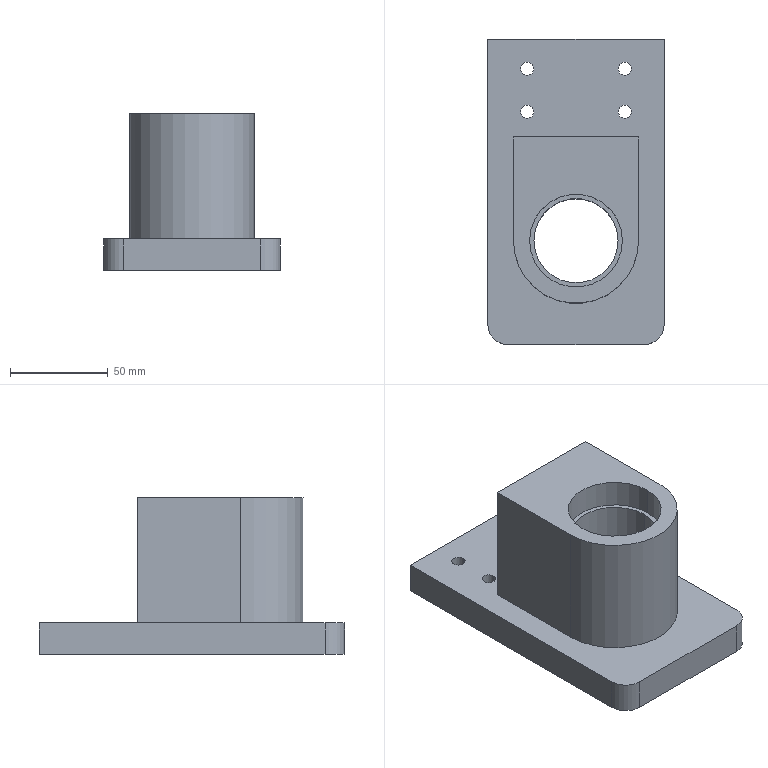NC program | NX | posted with a generic post | part box 90 x 156 x 80 mm
Lines 4832 to 5953 of 8711:
(CAVITY_MILL , TOOL : 刀杆C25-D25-150-2T)
N9656 T01 M6
N9658 G53
N9660 G17 G0 G90 X-99. Y0. S2000 M3
N9662 G43 Z30. H1
N9664 Z-38.5
N9666 G94 G1 Z-40.5 F3000.
N9668 X-82.75
N9670 Y48.792
N9672 X-82.741 Y50.037
N9674 G2 X-81.527 Y51.242 R1.214
N9676 G1 X81.527
N9678 G2 X82.741 Y50.036 R1.214
N9680 G1 X82.749 Y48.794
N9682 Y28.528
N9684 X64.029
N9686 G3 X60.769 Y32.522 R48.344
N9688 G1 X64.029
N9690 Y28.528
N9692 X70.622 Y17.418
N9694 X64.029 Y28.528
N9696 X82.749
N9698 X82.75 Y-48.792
N9700 X82.741 Y-50.037
N9702 G2 X81.527 Y-51.242 R1.214
N9704 G1 X60.769
N9706 Y-32.522
N9708 G3 X64.03 Y-28.527 R48.344
N9710 G1 X70.622 Y-17.417
N9712 X64.03 Y-28.527
N9714 Y-32.522
N9716 X60.769
N9718 Y-51.242
N9720 X-81.527
N9722 G2 X-82.741 Y-50.036 R1.214
N9724 G1 X-82.749 Y-48.794
N9726 X-82.75 Y0.
N9728 X-64.03
N9730 Y32.522
N9732 X-44.336
N9734 G3 X-44.344 Y32. R16.344
N9736 G1 Y-32.
N9738 G3 X-44.336 Y-32.522 R16.344
N9740 G1 X-40.594 Y-32.403
N9742 G2 X-40.6 Y-32. R12.6
N9744 G1 Y32.
N9746 G2 X-28. Y44.6 R12.6
N9748 G1 X25.
N9750 G2 X69.6 Y0. R44.6
N9752 X25. Y-44.6 R44.6
N9754 G1 X-28.
N9756 G2 X-40.594 Y-32.403 R12.6
N9758 G1 X-44.336 Y-32.522
N9760 X-64.029
N9762 X-64.03 Y0.
N9764 X-99.
N9766 Z-38.5
N9768 G0 Z30.
N9770 X33.853 Y-0.916
N9772 Z-37.
N9774 G2 X25. Y-8.9 Z-40.5 R8.9
N9776 X16.1 Y0. R8.9
N9778 X25. Y-8.9 R-8.9
N9780 G1 Z-38.5
N9782 G0 Z-37.5
N9784 X33.853 Y-0.916
N9786 G2 X25. Y-8.9 Z-41. R8.9
N9788 X16.1 Y0. R8.9
N9790 X25. Y-8.9 R-8.9
N9792 G1 Z-39.
N9794 G0 Z30.
N9796 X-99. Y0.
N9798 Z-39.
N9800 G1 Z-41.
N9802 X-82.75
N9804 Y48.792
N9806 X-82.741 Y50.037
N9808 G2 X-81.527 Y51.242 R1.214
N9810 G1 X81.527
N9812 G2 X82.741 Y50.036 R1.214
N9814 G1 X82.749 Y48.794
N9816 Y28.528
N9818 X64.029
N9820 G3 X60.769 Y32.522 R48.344
N9822 G1 X64.029
N9824 Y28.528
N9826 X70.622 Y17.418
N9828 X64.029 Y28.528
N9830 X82.749
N9832 X82.75 Y-48.792
N9834 X82.741 Y-50.037
N9836 G2 X81.527 Y-51.242 R1.214
N9838 G1 X60.769
N9840 Y-32.522
N9842 G3 X64.03 Y-28.527 R48.344
N9844 G1 X70.622 Y-17.417
N9846 X64.03 Y-28.527
N9848 Y-32.522
N9850 X60.769
N9852 Y-51.242
N9854 X-81.527
N9856 G2 X-82.741 Y-50.036 R1.214
N9858 G1 X-82.749 Y-48.794
N9860 X-82.75 Y0.
N9862 X-64.03
N9864 Y32.522
N9866 X-44.336
N9868 G3 X-44.344 Y32. R16.344
N9870 G1 Y-32.
N9872 G3 X-44.336 Y-32.522 R16.344
N9874 G1 X-40.594 Y-32.403
N9876 G2 X-40.6 Y-32. R12.6
N9878 G1 Y32.
N9880 G2 X-28. Y44.6 R12.6
N9882 G1 X25.
N9884 G2 X69.6 Y0. R44.6
N9886 X25. Y-44.6 R44.6
N9888 G1 X-28.
N9890 G2 X-40.594 Y-32.403 R12.6
N9892 G1 X-44.336 Y-32.522
N9894 X-64.029
N9896 X-64.03 Y0.
N9898 X-99.
N9900 Z-39.
N9902 G0 Z-38.5
N9904 Z-39.5
N9906 G1 Z-41.5
N9908 X-82.75
N9910 Y48.792
N9912 X-82.741 Y50.037
N9914 G2 X-81.527 Y51.242 R1.214
N9916 G1 X81.527
N9918 G2 X82.741 Y50.036 R1.214
N9920 G1 X82.749 Y48.794
N9922 Y28.528
N9924 X64.029
N9926 G3 X60.769 Y32.522 R48.344
N9928 G1 X64.029
N9930 Y28.528
N9932 X70.622 Y17.418
N9934 X64.029 Y28.528
N9936 X82.749
N9938 X82.75 Y-48.792
N9940 X82.741 Y-50.037
N9942 G2 X81.527 Y-51.242 R1.214
N9944 G1 X60.769
N9946 Y-32.522
N9948 G3 X64.03 Y-28.527 R48.344
N9950 G1 X70.622 Y-17.417
N9952 X64.03 Y-28.527
N9954 Y-32.522
N9956 X60.769
N9958 Y-51.242
N9960 X-81.527
N9962 G2 X-82.741 Y-50.036 R1.214
N9964 G1 X-82.749 Y-48.794
N9966 X-82.75 Y0.
N9968 X-64.03
N9970 Y32.522
N9972 X-44.336
N9974 G3 X-44.344 Y32. R16.344
N9976 G1 Y-32.
N9978 G3 X-44.336 Y-32.522 R16.344
N9980 G1 X-40.594 Y-32.403
N9982 G2 X-40.6 Y-32. R12.6
N9984 G1 Y32.
N9986 G2 X-28. Y44.6 R12.6
N9988 G1 X25.
N9990 G2 X69.6 Y0. R44.6
N9992 X25. Y-44.6 R44.6
N9994 G1 X-28.
N9996 G2 X-40.594 Y-32.403 R12.6
N9998 G1 X-44.336 Y-32.522
N10000 X-64.029
N10002 X-64.03 Y0.
N10004 X-99.
N10006 Z-39.5
N10008 G0 Z30.
N10010 X33.853 Y-0.916
N10012 Z-38.
N10014 G2 X25. Y-8.9 Z-41.5 R8.9
N10016 X16.1 Y0. R8.9
N10018 X25. Y-8.9 R-8.9
N10020 G1 Z-39.5
N10022 G0 Z-38.5
N10024 X33.853 Y-0.916
N10026 G2 X25. Y-8.9 Z-42. R8.9
N10028 X16.1 Y0. R8.9
N10030 X25. Y-8.9 R-8.9
N10032 G1 Z-40.
N10034 G0 Z30.
N10036 X-99. Y0.
N10038 Z-40.
N10040 G1 Z-42.
N10042 X-82.75
N10044 Y48.792
N10046 X-82.741 Y50.037
N10048 G2 X-81.527 Y51.242 R1.214
N10050 G1 X81.527
N10052 G2 X82.741 Y50.036 R1.214
N10054 G1 X82.749 Y48.794
N10056 Y28.528
N10058 X64.029
N10060 G3 X60.769 Y32.522 R48.344
N10062 G1 X64.029
N10064 Y28.528
N10066 X70.622 Y17.418
N10068 X64.029 Y28.528
N10070 X82.749
N10072 X82.75 Y-48.792
N10074 X82.741 Y-50.037
N10076 G2 X81.527 Y-51.242 R1.214
N10078 G1 X60.769
N10080 Y-32.522
N10082 G3 X64.03 Y-28.527 R48.344
N10084 G1 X70.622 Y-17.417
N10086 X64.03 Y-28.527
N10088 Y-32.522
N10090 X60.769
N10092 Y-51.242
N10094 X-81.527
N10096 G2 X-82.741 Y-50.036 R1.214
N10098 G1 X-82.749 Y-48.794
N10100 X-82.75 Y0.
N10102 X-64.03
N10104 Y32.522
N10106 X-44.336
N10108 G3 X-44.344 Y32. R16.344
N10110 G1 Y-32.
N10112 G3 X-44.336 Y-32.522 R16.344
N10114 G1 X-40.594 Y-32.403
N10116 G2 X-40.6 Y-32. R12.6
N10118 G1 Y32.
N10120 G2 X-28. Y44.6 R12.6
N10122 G1 X25.
N10124 G2 X69.6 Y0. R44.6
N10126 X25. Y-44.6 R44.6
N10128 G1 X-28.
N10130 G2 X-40.594 Y-32.403 R12.6
N10132 G1 X-44.336 Y-32.522
N10134 X-64.029
N10136 X-64.03 Y0.
N10138 X-99.
N10140 Z-40.
N10142 G0 Z-39.5
N10144 Z-40.5
N10146 G1 Z-42.5
N10148 X-82.75
N10150 Y48.792
N10152 X-82.741 Y50.037
N10154 G2 X-81.527 Y51.242 R1.214
N10156 G1 X81.527
N10158 G2 X82.741 Y50.036 R1.214
N10160 G1 X82.749 Y48.794
N10162 Y28.528
N10164 X64.029
N10166 G3 X60.769 Y32.522 R48.344
N10168 G1 X64.029
N10170 Y28.528
N10172 X70.622 Y17.418
N10174 X64.029 Y28.528
N10176 X82.749
N10178 X82.75 Y-48.792
N10180 X82.741 Y-50.037
N10182 G2 X81.527 Y-51.242 R1.214
N10184 G1 X60.769
N10186 Y-32.522
N10188 G3 X64.03 Y-28.527 R48.344
N10190 G1 X70.622 Y-17.417
N10192 X64.03 Y-28.527
N10194 Y-32.522
N10196 X60.769
N10198 Y-51.242
N10200 X-81.527
N10202 G2 X-82.741 Y-50.036 R1.214
N10204 G1 X-82.749 Y-48.794
N10206 X-82.75 Y0.
N10208 X-64.03
N10210 Y32.522
N10212 X-44.336
N10214 G3 X-44.344 Y32. R16.344
N10216 G1 Y-32.
N10218 G3 X-44.336 Y-32.522 R16.344
N10220 G1 X-40.594 Y-32.403
N10222 G2 X-40.6 Y-32. R12.6
N10224 G1 Y32.
N10226 G2 X-28. Y44.6 R12.6
N10228 G1 X25.
N10230 G2 X69.6 Y0. R44.6
N10232 X25. Y-44.6 R44.6
N10234 G1 X-28.
N10236 G2 X-40.594 Y-32.403 R12.6
N10238 G1 X-44.336 Y-32.522
N10240 X-64.029
N10242 X-64.03 Y0.
N10244 X-99.
N10246 Z-40.5
N10248 G0 Z30.
N10250 X33.853 Y-0.916
N10252 Z-39.
N10254 G2 X25. Y-8.9 Z-42.5 R8.9
N10256 X16.1 Y0. R8.9
N10258 X25. Y-8.9 R-8.9
N10260 G1 Z-40.5
N10262 G0 Z-39.5
N10264 X33.853 Y-0.916
N10266 G2 X25. Y-8.9 Z-43. R8.9
N10268 X16.1 Y0. R8.9
N10270 X25. Y-8.9 R-8.9
N10272 G1 Z-41.
N10274 G0 Z30.
N10276 X-99. Y0.
N10278 Z-41.
N10280 G1 Z-43.
N10282 X-82.75
N10284 Y48.792
N10286 X-82.741 Y50.037
N10288 G2 X-81.527 Y51.242 R1.214
N10290 G1 X81.527
N10292 G2 X82.741 Y50.036 R1.214
N10294 G1 X82.749 Y48.794
N10296 Y28.528
N10298 X64.029
N10300 G3 X60.769 Y32.522 R48.344
N10302 G1 X64.029
N10304 Y28.528
N10306 X70.622 Y17.418
N10308 X64.029 Y28.528
N10310 X82.749
N10312 X82.75 Y-48.792
N10314 X82.741 Y-50.037
N10316 G2 X81.527 Y-51.242 R1.214
N10318 G1 X60.769
N10320 Y-32.522
N10322 G3 X64.03 Y-28.527 R48.344
N10324 G1 X70.622 Y-17.417
N10326 X64.03 Y-28.527
N10328 Y-32.522
N10330 X60.769
N10332 Y-51.242
N10334 X-81.527
N10336 G2 X-82.741 Y-50.036 R1.214
N10338 G1 X-82.749 Y-48.794
N10340 X-82.75 Y0.
N10342 X-64.03
N10344 Y32.522
N10346 X-44.336
N10348 G3 X-44.344 Y32. R16.344
N10350 G1 Y-32.
N10352 G3 X-44.336 Y-32.522 R16.344
N10354 G1 X-40.594 Y-32.403
N10356 G2 X-40.6 Y-32. R12.6
N10358 G1 Y32.
N10360 G2 X-28. Y44.6 R12.6
N10362 G1 X25.
N10364 G2 X69.6 Y0. R44.6
N10366 X25. Y-44.6 R44.6
N10368 G1 X-28.
N10370 G2 X-40.594 Y-32.403 R12.6
N10372 G1 X-44.336 Y-32.522
N10374 X-64.029
N10376 X-64.03 Y0.
N10378 X-99.
N10380 Z-41.
N10382 G0 Z-40.5
N10384 Z-41.5
N10386 G1 Z-43.5
N10388 X-82.75
N10390 Y48.792
N10392 X-82.741 Y50.037
N10394 G2 X-81.527 Y51.242 R1.214
N10396 G1 X81.527
N10398 G2 X82.741 Y50.036 R1.214
N10400 G1 X82.749 Y48.794
N10402 X82.75 Y28.528
N10404 X64.03
N10406 G3 X60.769 Y32.522 R48.344
N10408 G1 X64.029
N10410 X64.03 Y28.528
N10412 X70.622 Y17.418
N10414 X64.03 Y28.528
N10416 X82.75
N10418 Y-48.792
N10420 X82.741 Y-50.037
N10422 G2 X81.527 Y-51.242 R1.214
N10424 G1 X60.769
N10426 Y-32.522
N10428 G3 X64.03 Y-28.527 R48.344
N10430 G1 X70.622 Y-17.417
N10432 X64.03 Y-28.527
N10434 Y-32.522
N10436 X60.769
N10438 Y-51.242
N10440 X-81.527
N10442 G2 X-82.741 Y-50.036 R1.214
N10444 G1 X-82.749 Y-48.794
N10446 X-82.75 Y0.
N10448 X-64.03
N10450 Y32.522
N10452 X-44.336
N10454 G3 X-44.344 Y32. R16.344
N10456 G1 Y-32.
N10458 G3 X-44.336 Y-32.522 R16.344
N10460 G1 X-40.594 Y-32.403
N10462 G2 X-40.6 Y-32. R12.6
N10464 G1 Y32.
N10466 G2 X-28. Y44.6 R12.6
N10468 G1 X25.
N10470 G2 X69.6 Y0. R44.6
N10472 X25. Y-44.6 R44.6
N10474 G1 X-28.
N10476 G2 X-40.594 Y-32.403 R12.6
N10478 G1 X-44.336 Y-32.522
N10480 X-64.029
N10482 X-64.03 Y0.
N10484 X-99.
N10486 Z-41.5
N10488 G0 Z30.
N10490 X33.853 Y-0.916
N10492 Z-40.
N10494 G2 X25. Y-8.9 Z-43.5 R8.9
N10496 X16.1 Y0. R8.9
N10498 X25. Y-8.9 R-8.9
N10500 G1 Z-41.5
N10502 G0 Z-40.5
N10504 X33.853 Y-0.916
N10506 G2 X25. Y-8.9 Z-44. R8.9
N10508 X16.1 Y0. R8.9
N10510 X25. Y-8.9 R-8.9
N10512 G1 Z-42.
N10514 G0 Z30.
N10516 X-99. Y0.
N10518 Z-42.
N10520 G1 Z-44.
N10522 X-82.75
N10524 Y48.792
N10526 X-82.741 Y50.037
N10528 G2 X-81.527 Y51.242 R1.214
N10530 G1 X81.527
N10532 G2 X82.741 Y50.036 R1.214
N10534 G1 X82.749 Y48.794
N10536 X82.75 Y28.528
N10538 X64.03
N10540 G3 X60.769 Y32.522 R48.344
N10542 G1 X64.029
N10544 X64.03 Y28.528
N10546 X70.622 Y17.418
N10548 X64.03 Y28.528
N10550 X82.75
N10552 Y-48.792
N10554 X82.741 Y-50.037
N10556 G2 X81.527 Y-51.242 R1.214
N10558 G1 X60.769
N10560 Y-32.522
N10562 G3 X64.03 Y-28.527 R48.344
N10564 G1 X70.622 Y-17.417
N10566 X64.03 Y-28.527
N10568 Y-32.522
N10570 X60.769
N10572 Y-51.242
N10574 X-81.527
N10576 G2 X-82.741 Y-50.036 R1.214
N10578 G1 X-82.749 Y-48.794
N10580 X-82.75 Y0.
N10582 X-64.03
N10584 Y32.522
N10586 X-44.336
N10588 G3 X-44.344 Y32. R16.344
N10590 G1 Y-32.
N10592 G3 X-44.336 Y-32.522 R16.344
N10594 G1 X-40.594 Y-32.403
N10596 G2 X-40.6 Y-32. R12.6
N10598 G1 Y32.
N10600 G2 X-28. Y44.6 R12.6
N10602 G1 X25.
N10604 G2 X69.6 Y0. R44.6
N10606 X25. Y-44.6 R44.6
N10608 G1 X-28.
N10610 G2 X-40.594 Y-32.403 R12.6
N10612 G1 X-44.336 Y-32.522
N10614 X-64.029
N10616 X-64.03 Y0.
N10618 X-99.
N10620 Z-42.
N10622 G0 Z-41.5
N10624 Z-42.5
N10626 G1 Z-44.5
N10628 X-82.75
N10630 Y48.792
N10632 X-82.741 Y50.037
N10634 G2 X-81.527 Y51.242 R1.214
N10636 G1 X81.527
N10638 G2 X82.741 Y50.036 R1.214
N10640 G1 X82.749 Y48.794
N10642 X82.75 Y28.528
N10644 X64.03
N10646 G3 X60.769 Y32.522 R48.344
N10648 G1 X64.029
N10650 X64.03 Y28.528
N10652 X70.622 Y17.418
N10654 X64.03 Y28.528
N10656 X82.75
N10658 Y-48.792
N10660 X82.741 Y-50.037
N10662 G2 X81.527 Y-51.242 R1.214
N10664 G1 X60.769
N10666 Y-32.522
N10668 G3 X64.03 Y-28.527 R48.344
N10670 G1 X70.622 Y-17.417
N10672 X64.03 Y-28.527
N10674 Y-32.522
N10676 X60.769
N10678 Y-51.242
N10680 X-81.527
N10682 G2 X-82.741 Y-50.036 R1.214
N10684 G1 X-82.749 Y-48.794
N10686 X-82.75 Y0.
N10688 X-64.03
N10690 Y32.522
N10692 X-44.336
N10694 G3 X-44.344 Y32. R16.344
N10696 G1 Y-32.
N10698 G3 X-44.336 Y-32.522 R16.344
N10700 G1 X-40.594 Y-32.403
N10702 G2 X-40.6 Y-32. R12.6
N10704 G1 Y32.
N10706 G2 X-28. Y44.6 R12.6
N10708 G1 X25.
N10710 G2 X69.6 Y0. R44.6
N10712 X25. Y-44.6 R44.6
N10714 G1 X-28.
N10716 G2 X-40.594 Y-32.403 R12.6
N10718 G1 X-44.336 Y-32.522
N10720 X-64.029
N10722 X-64.03 Y0.
N10724 X-99.
N10726 Z-42.5
N10728 G0 Z30.
N10730 X33.853 Y-0.916
N10732 Z-41.
N10734 G2 X25. Y-8.9 Z-44.5 R8.9
N10736 X16.1 Y0. R8.9
N10738 X25. Y-8.9 R-8.9
N10740 G1 Z-42.5
N10742 G0 Z-41.5
N10744 X33.853 Y-0.916
N10746 G2 X25. Y-8.9 Z-45. R8.9
N10748 X16.1 Y0. R8.9
N10750 X25. Y-8.9 R-8.9
N10752 G1 Z-43.
N10754 G0 Z30.
N10756 X-99. Y0.
N10758 Z-43.
N10760 G1 Z-45.
N10762 X-82.75
N10764 Y48.792
N10766 X-82.741 Y50.037
N10768 G2 X-81.527 Y51.242 R1.214
N10770 G1 X81.527
N10772 G2 X82.741 Y50.036 R1.214
N10774 G1 X82.749 Y48.794
N10776 X82.75 Y28.528
N10778 X64.03
N10780 G3 X60.769 Y32.522 R48.344
N10782 G1 X64.029
N10784 X64.03 Y28.528
N10786 X70.622 Y17.418
N10788 X64.03 Y28.528
N10790 X82.75
N10792 Y-48.792
N10794 X82.741 Y-50.037
N10796 G2 X81.527 Y-51.242 R1.214
N10798 G1 X60.769
N10800 Y-32.522
N10802 G3 X64.03 Y-28.527 R48.344
N10804 G1 X70.622 Y-17.417
N10806 X64.03 Y-28.527
N10808 Y-32.522
N10810 X60.769
N10812 Y-51.242
N10814 X-81.527
N10816 G2 X-82.741 Y-50.036 R1.214
N10818 G1 X-82.749 Y-48.794
N10820 X-82.75 Y0.
N10822 X-64.03
N10824 Y32.522
N10826 X-44.336
N10828 G3 X-44.344 Y32. R16.344
N10830 G1 Y-32.
N10832 G3 X-44.336 Y-32.522 R16.344
N10834 G1 X-40.594 Y-32.403
N10836 G2 X-40.6 Y-32. R12.6
N10838 G1 Y32.
N10840 G2 X-28. Y44.6 R12.6
N10842 G1 X25.
N10844 G2 X69.6 Y0. R44.6
N10846 X25. Y-44.6 R44.6
N10848 G1 X-28.
N10850 G2 X-40.594 Y-32.403 R12.6
N10852 G1 X-44.336 Y-32.522
N10854 X-64.029
N10856 X-64.03 Y0.
N10858 X-99.
N10860 Z-43.
N10862 G0 Z-42.5
N10864 Z-43.5
N10866 G1 Z-45.5
N10868 X-82.75
N10870 Y48.792
N10872 X-82.741 Y50.037
N10874 G2 X-81.527 Y51.242 R1.214
N10876 G1 X81.527
N10878 G2 X82.741 Y50.036 R1.214
N10880 G1 X82.749 Y48.794
N10882 X82.75 Y28.528
N10884 X64.03
N10886 G3 X60.769 Y32.522 R48.344
N10888 G1 X64.029
N10890 X64.03 Y28.528
N10892 X70.622 Y17.418
N10894 X64.03 Y28.528
N10896 X82.75
N10898 Y-48.792
N10900 X82.741 Y-50.037
N10902 G2 X81.527 Y-51.242 R1.214
N10904 G1 X60.769
N10906 Y-32.522
N10908 G3 X64.03 Y-28.527 R48.344
N10910 G1 X70.622 Y-17.417
N10912 X64.03 Y-28.527
N10914 Y-32.522
N10916 X60.769
N10918 Y-51.242
N10920 X-81.527
N10922 G2 X-82.741 Y-50.036 R1.214
N10924 G1 X-82.749 Y-48.794
N10926 X-82.75 Y0.
N10928 X-64.03
N10930 Y32.522
N10932 X-44.336
N10934 G3 X-44.344 Y32. R16.344
N10936 G1 Y-32.
N10938 G3 X-44.336 Y-32.522 R16.344
N10940 G1 X-40.594 Y-32.403
N10942 G2 X-40.6 Y-32. R12.6
N10944 G1 Y32.
N10946 G2 X-28. Y44.6 R12.6
N10948 G1 X25.
N10950 G2 X69.6 Y0. R44.6
N10952 X25. Y-44.6 R44.6
N10954 G1 X-28.
N10956 G2 X-40.594 Y-32.403 R12.6
N10958 G1 X-44.336 Y-32.522
N10960 X-64.029
N10962 X-64.03 Y0.
N10964 X-99.
N10966 Z-43.5
N10968 G0 Z30.
N10970 X33.853 Y-0.916
N10972 Z-42.
N10974 G2 X25. Y-8.9 Z-45.5 R8.9
N10976 X16.1 Y0. R8.9
N10978 X25. Y-8.9 R-8.9
N10980 G1 Z-43.5
N10982 G0 Z-42.5
N10984 X33.853 Y-0.916
N10986 G2 X25. Y-8.9 Z-46. R8.9
N10988 X16.1 Y0. R8.9
N10990 X25. Y-8.9 R-8.9
N10992 G1 Z-44.
N10994 G0 Z30.
N10996 X-99. Y0.
N10998 Z-44.
N11000 G1 Z-46.
N11002 X-82.75
N11004 Y48.792
N11006 X-82.741 Y50.037
N11008 G2 X-81.527 Y51.242 R1.214
N11010 G1 X81.527
N11012 G2 X82.741 Y50.036 R1.214
N11014 G1 X82.749 Y48.794
N11016 X82.75 Y28.528
N11018 X64.03
N11020 G3 X60.769 Y32.522 R48.344
N11022 G1 X64.03
N11024 Y28.528
N11026 X70.622 Y17.418
N11028 X64.03 Y28.528
N11030 X82.75
N11032 Y-48.792
N11034 X82.741 Y-50.037
N11036 G2 X81.527 Y-51.242 R1.214
N11038 G1 X60.769
N11040 Y-32.522
N11042 G3 X64.03 Y-28.527 R48.344
N11044 G1 X70.622 Y-17.417
N11046 X64.03 Y-28.527
N11048 Y-32.522
N11050 X60.769
N11052 Y-51.242
N11054 X-81.527
N11056 G2 X-82.741 Y-50.036 R1.214
N11058 G1 X-82.749 Y-48.794
N11060 X-82.75 Y0.
N11062 X-64.03
N11064 Y32.522
N11066 X-44.336
N11068 G3 X-44.344 Y32. R16.344
N11070 G1 Y-32.
N11072 G3 X-44.336 Y-32.522 R16.344
N11074 G1 X-40.594 Y-32.403
N11076 G2 X-40.6 Y-32. R12.6
N11078 G1 Y32.
N11080 G2 X-28. Y44.6 R12.6
N11082 G1 X25.
N11084 G2 X69.6 Y0. R44.6
N11086 X25. Y-44.6 R44.6
N11088 G1 X-28.
N11090 G2 X-40.594 Y-32.403 R12.6
N11092 G1 X-44.336 Y-32.522
N11094 X-64.03
N11096 Y0.
N11098 X-99.
N11100 Z-44.
N11102 G0 Z-43.5
N11104 Z-44.5
N11106 G1 Z-46.5
N11108 X-82.75
N11110 Y48.792
N11112 X-82.741 Y50.037
N11114 G2 X-81.527 Y51.242 R1.214
N11116 G1 X81.527
N11118 G2 X82.741 Y50.036 R1.214
N11120 G1 X82.749 Y48.794
N11122 X82.75 Y28.528
N11124 X64.03
N11126 G3 X60.769 Y32.522 R48.344
N11128 G1 X64.03
N11130 Y28.528
N11132 X70.622 Y17.418
N11134 X64.03 Y28.528
N11136 X82.75
N11138 Y-48.792
N11140 X82.741 Y-50.037
N11142 G2 X81.527 Y-51.242 R1.214
N11144 G1 X60.769
N11146 Y-32.522
N11148 G3 X64.03 Y-28.527 R48.344
N11150 G1 X70.622 Y-17.417
N11152 X64.03 Y-28.527
N11154 Y-32.522
N11156 X60.769
N11158 Y-51.242
N11160 X-81.527
N11162 G2 X-82.741 Y-50.036 R1.214
N11164 G1 X-82.749 Y-48.794
N11166 X-82.75 Y0.
N11168 X-64.03
N11170 Y32.522
N11172 X-44.336
N11174 G3 X-44.344 Y32. R16.344
N11176 G1 Y-32.
N11178 G3 X-44.336 Y-32.522 R16.344
N11180 G1 X-40.594 Y-32.403
N11182 G2 X-40.6 Y-32. R12.6
N11184 G1 Y32.
N11186 G2 X-28. Y44.6 R12.6
N11188 G1 X25.
N11190 G2 X69.6 Y0. R44.6
N11192 X25. Y-44.6 R44.6
N11194 G1 X-28.
N11196 G2 X-40.594 Y-32.403 R12.6
N11198 G1 X-44.336 Y-32.522
N11200 X-64.03
N11202 Y0.
N11204 X-99.
N11206 Z-44.5
N11208 G0 Z30.
N11210 X33.853 Y-0.916
N11212 Z-43.
N11214 G2 X25. Y-8.9 Z-46.5 R8.9
N11216 X16.1 Y0. R8.9
N11218 X25. Y-8.9 R-8.9
N11220 G1 Z-44.5
N11222 G0 Z-43.5
N11224 X33.853 Y-0.916
N11226 G2 X25. Y-8.9 Z-47. R8.9
N11228 X16.1 Y0. R8.9
N11230 X25. Y-8.9 R-8.9
N11232 G1 Z-45.
N11234 G0 Z30.
N11236 X-99. Y0.
N11238 Z-45.
N11240 G1 Z-47.
N11242 X-82.75
N11244 Y48.792
N11246 X-82.741 Y50.037
N11248 G2 X-81.527 Y51.242 R1.214
N11250 G1 X81.527
N11252 G2 X82.741 Y50.036 R1.214
N11254 G1 X82.749 Y48.794
N11256 X82.75 Y28.528
N11258 X64.03
N11260 G3 X60.769 Y32.522 R48.344
N11262 G1 X64.03
N11264 Y28.528
N11266 X70.622 Y17.418
N11268 X64.03 Y28.528
N11270 X82.75
N11272 Y-48.792
N11274 X82.741 Y-50.037
N11276 G2 X81.527 Y-51.242 R1.214
N11278 G1 X60.769
N11280 Y-32.522
N11282 G3 X64.03 Y-28.527 R48.344
N11284 G1 X70.622 Y-17.417
N11286 X64.03 Y-28.527
N11288 Y-32.522
N11290 X60.769
N11292 Y-51.242
N11294 X-81.527
N11296 G2 X-82.741 Y-50.036 R1.214
N11298 G1 X-82.749 Y-48.794
N11300 X-82.75 Y0.
N11302 X-64.03
N11304 Y32.522
N11306 X-44.336
N11308 G3 X-44.344 Y32. R16.344
N11310 G1 Y-32.
N11312 G3 X-44.336 Y-32.522 R16.344
N11314 G1 X-40.594 Y-32.403
N11316 G2 X-40.6 Y-32. R12.6
N11318 G1 Y32.
N11320 G2 X-28. Y44.6 R12.6
N11322 G1 X25.
N11324 G2 X69.6 Y0. R44.6
N11326 X25. Y-44.6 R44.6
N11328 G1 X-28.
N11330 G2 X-40.594 Y-32.403 R12.6
N11332 G1 X-44.336 Y-32.522
N11334 X-64.03
N11336 Y0.
N11338 X-99.
N11340 Z-45.
N11342 G0 Z-44.5
N11344 Z-45.5
N11346 G1 Z-47.5
N11348 X-82.75
N11350 Y48.792
N11352 X-82.741 Y50.037
N11354 G2 X-81.527 Y51.242 R1.214
N11356 G1 X81.527
N11358 G2 X82.741 Y50.036 R1.214
N11360 G1 X82.749 Y48.794
N11362 X82.75 Y28.528
N11364 X64.03
N11366 G3 X60.769 Y32.522 R48.344
N11368 G1 X64.03
N11370 Y28.528
N11372 X70.622 Y17.418
N11374 X64.03 Y28.528
N11376 X82.75
N11378 Y-48.792
N11380 X82.741 Y-50.037
N11382 G2 X81.527 Y-51.242 R1.214
N11384 G1 X60.769
N11386 Y-32.522
N11388 G3 X64.03 Y-28.527 R48.344
N11390 G1 X70.622 Y-17.417
N11392 X64.03 Y-28.527
N11394 Y-32.522
N11396 X60.769
N11398 Y-51.242
N11400 X-81.527
N11402 G2 X-82.741 Y-50.036 R1.214
N11404 G1 X-82.749 Y-48.794
N11406 X-82.75 Y0.
N11408 X-64.03
N11410 Y32.522
N11412 X-44.336
N11414 G3 X-44.344 Y32. R16.344
N11416 G1 Y-32.
N11418 G3 X-44.336 Y-32.522 R16.344
N11420 G1 X-40.594 Y-32.403
N11422 G2 X-40.6 Y-32. R12.6
N11424 G1 Y32.
N11426 G2 X-28. Y44.6 R12.6
N11428 G1 X25.
N11430 G2 X69.6 Y0. R44.6
N11432 X25. Y-44.6 R44.6
N11434 G1 X-28.
N11436 G2 X-40.594 Y-32.403 R12.6
N11438 G1 X-44.336 Y-32.522
N11440 X-64.03
N11442 Y0.
N11444 X-99.
N11446 Z-45.5
N11448 G0 Z30.
N11450 X33.853 Y-0.916
N11452 Z-44.
N11454 G2 X25. Y-8.9 Z-47.5 R8.9
N11456 X16.1 Y0. R8.9
N11458 X25. Y-8.9 R-8.9
N11460 G1 Z-45.5
N11462 G0 Z-44.5
N11464 X33.853 Y-0.916
N11466 G2 X25. Y-8.9 Z-48. R8.9
N11468 X16.1 Y0. R8.9
N11470 X25. Y-8.9 R-8.9
N11472 G1 Z-46.
N11474 G0 Z30.
N11476 X-99. Y0.
N11478 Z-46.
N11480 G1 Z-48.
N11482 X-82.75
N11484 Y48.792
N11486 X-82.741 Y50.037
N11488 G2 X-81.527 Y51.242 R1.214
N11490 G1 X81.527
N11492 G2 X82.741 Y50.036 R1.214
N11494 G1 X82.749 Y48.794
N11496 X82.75 Y28.528
N11498 X64.03
N11500 G3 X60.769 Y32.522 R48.344
N11502 G1 X64.03
N11504 Y28.528
N11506 X70.622 Y17.418
N11508 X64.03 Y28.528
N11510 X82.75
N11512 Y-48.792
N11514 X82.741 Y-50.037
N11516 G2 X81.527 Y-51.242 R1.214
N11518 G1 X60.769
N11520 Y-32.522
N11522 G3 X64.03 Y-28.527 R48.344
N11524 G1 X70.622 Y-17.417
N11526 X64.03 Y-28.527
N11528 Y-32.522
N11530 X60.769
N11532 Y-51.242
N11534 X-81.527
N11536 G2 X-82.741 Y-50.036 R1.214
N11538 G1 X-82.749 Y-48.794
N11540 X-82.75 Y0.
N11542 X-64.03
N11544 Y32.522
N11546 X-44.336
N11548 G3 X-44.344 Y32. R16.344
N11550 G1 Y-32.
N11552 G3 X-44.336 Y-32.522 R16.344
N11554 G1 X-40.594 Y-32.403
N11556 G2 X-40.6 Y-32. R12.6
N11558 G1 Y32.
N11560 G2 X-28. Y44.6 R12.6
N11562 G1 X25.
N11564 G2 X69.6 Y0. R44.6
N11566 X25. Y-44.6 R44.6
N11568 G1 X-28.
N11570 G2 X-40.594 Y-32.403 R12.6
N11572 G1 X-44.336 Y-32.522
N11574 X-64.03
N11576 Y0.
N11578 X-99.
N11580 Z-46.
N11582 G0 Z-45.5
N11584 Z-46.5
N11586 G1 Z-48.5
N11588 X-82.75
N11590 Y48.792
N11592 X-82.741 Y50.037
N11594 G2 X-81.527 Y51.242 R1.214
N11596 G1 X81.527
N11598 G2 X82.741 Y50.036 R1.214
N11600 G1 X82.749 Y48.794
N11602 X82.75 Y28.528
N11604 X64.03
N11606 G3 X60.769 Y32.522 R48.344
N11608 G1 X64.03
N11610 Y28.528
N11612 X70.622 Y17.418
N11614 X64.03 Y28.528
N11616 X82.75
N11618 Y-48.792
N11620 X82.741 Y-50.037
N11622 G2 X81.527 Y-51.242 R1.214
N11624 G1 X60.769
N11626 Y-32.522
N11628 G3 X64.03 Y-28.527 R48.344
N11630 G1 X70.622 Y-17.417
N11632 X64.03 Y-28.527
N11634 Y-32.522
N11636 X60.769
N11638 Y-51.242
N11640 X-81.527
N11642 G2 X-82.741 Y-50.036 R1.214
N11644 G1 X-82.749 Y-48.794
N11646 X-82.75 Y0.
N11648 X-64.03
N11650 Y32.522
N11652 X-44.336
N11654 G3 X-44.344 Y32. R16.344
N11656 G1 Y-32.
N11658 G3 X-44.336 Y-32.522 R16.344
N11660 G1 X-40.594 Y-32.403
N11662 G2 X-40.6 Y-32. R12.6
N11664 G1 Y32.
N11666 G2 X-28. Y44.6 R12.6
N11668 G1 X25.
N11670 G2 X69.6 Y0. R44.6
N11672 X25. Y-44.6 R44.6
N11674 G1 X-28.
N11676 G2 X-40.594 Y-32.403 R12.6
N11678 G1 X-44.336 Y-32.522
N11680 X-64.03
N11682 Y0.
N11684 X-99.
N11686 Z-46.5
N11688 G0 Z30.
N11690 X33.853 Y-0.916
N11692 Z-45.
N11694 G2 X25. Y-8.9 Z-48.5 R8.9
N11696 X16.1 Y0. R8.9
N11698 X25. Y-8.9 R-8.9
N11700 G1 Z-46.5
N11702 G0 Z-45.5
N11704 X33.853 Y-0.916
N11706 G2 X25. Y-8.9 Z-49. R8.9
N11708 X16.1 Y0. R8.9
N11710 X25. Y-8.9 R-8.9
N11712 G1 Z-47.
N11714 G0 Z30.
N11716 X-99. Y0.
N11718 Z-47.
N11720 G1 Z-49.
N11722 X-82.75
N11724 Y48.792
N11726 X-82.741 Y50.037
N11728 G2 X-81.527 Y51.242 R1.214
N11730 G1 X81.527
N11732 G2 X82.741 Y50.036 R1.214
N11734 G1 X82.749 Y48.794
N11736 X82.75 Y28.528
N11738 X64.03
N11740 G3 X60.769 Y32.522 R48.344
N11742 G1 X64.03
N11744 Y28.528
N11746 X70.622 Y17.418
N11748 X64.03 Y28.528
N11750 X82.75
N11752 Y-48.792
N11754 X82.741 Y-50.037
N11756 G2 X81.527 Y-51.242 R1.214
N11758 G1 X60.769
N11760 Y-32.522
N11762 G3 X64.03 Y-28.527 R48.344
N11764 G1 X70.622 Y-17.417
N11766 X64.03 Y-28.527
N11768 Y-32.522
N11770 X60.769
N11772 Y-51.242
N11774 X-81.527
N11776 G2 X-82.741 Y-50.036 R1.214
N11778 G1 X-82.749 Y-48.794
N11780 X-82.75 Y0.
N11782 X-64.03
N11784 Y32.522
N11786 X-44.336
N11788 G3 X-44.344 Y32. R16.344
N11790 G1 Y-32.
N11792 G3 X-44.336 Y-32.522 R16.344
N11794 G1 X-40.594 Y-32.403
N11796 G2 X-40.6 Y-32. R12.6
N11798 G1 Y32.
N11800 G2 X-28. Y44.6 R12.6
N11802 G1 X25.
N11804 G2 X69.6 Y0. R44.6
N11806 X25. Y-44.6 R44.6
N11808 G1 X-28.
N11810 G2 X-40.594 Y-32.403 R12.6
N11812 G1 X-44.336 Y-32.522
N11814 X-64.03
N11816 Y0.
N11818 X-99.
N11820 Z-47.
N11822 G0 Z-46.5
N11824 Z-47.5
N11826 G1 Z-49.5
N11828 X-82.75
N11830 Y48.792
N11832 X-82.741 Y50.037
N11834 G2 X-81.527 Y51.242 R1.214
N11836 G1 X81.527
N11838 G2 X82.741 Y50.036 R1.214
N11840 G1 X82.749 Y48.794
N11842 X82.75 Y28.528
N11844 X64.03
N11846 G3 X60.769 Y32.522 R48.344
N11848 G1 X64.03
N11850 Y28.528
N11852 X70.622 Y17.418
N11854 X64.03 Y28.528
N11856 X82.75
N11858 Y-48.792
N11860 X82.741 Y-50.037
N11862 G2 X81.527 Y-51.242 R1.214
N11864 G1 X60.769
N11866 Y-32.522
N11868 G3 X64.03 Y-28.527 R48.344
N11870 G1 X70.622 Y-17.417
N11872 X64.03 Y-28.527
N11874 Y-32.522
N11876 X60.769
N11878 Y-51.242
N11880 X-81.527
N11882 G2 X-82.741 Y-50.036 R1.214
N11884 G1 X-82.749 Y-48.794
N11886 X-82.75 Y0.
N11888 X-64.03
N11890 Y32.522
N11892 X-44.336